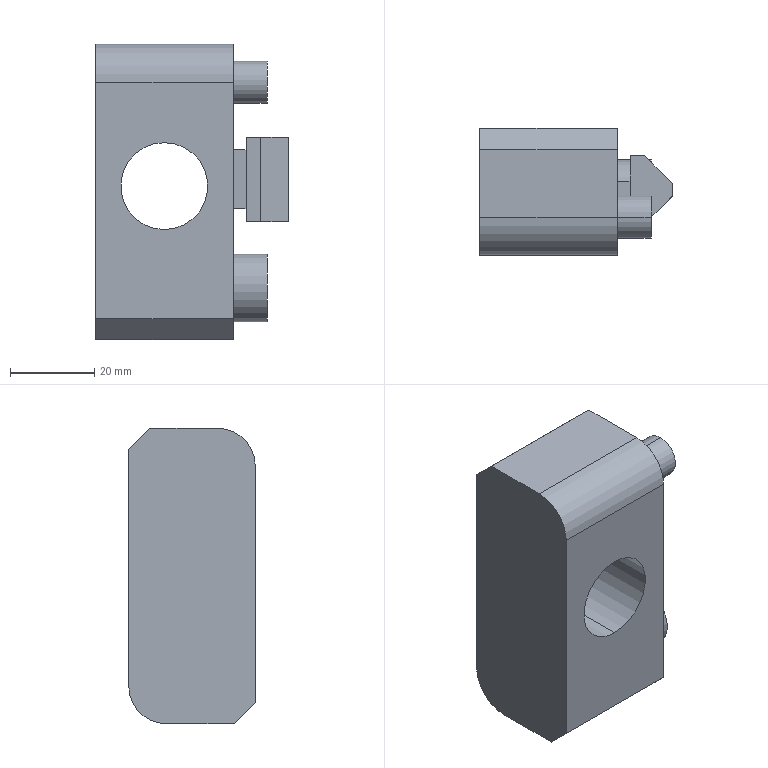Part | SolidWorks | features BaseBody 1 | 1 solid | 30 faces | box 45.6 x 30 x 70 mm | volume 61273 mm3 | plane 22 | cylinder 8 | commonest cylinder face diameters 10 x2 16 x2 18 x2 20.6 x2
STEP:
#1=CARTESIAN_POINT('',(-215.391,-172.8,1136.061));
#2=VERTEX_POINT('',#1);
#3=CARTESIAN_POINT('',(-215.391,-172.8,1126.061));
#4=VERTEX_POINT('',#3);
#5=CARTESIAN_POINT('',(-215.391,-172.8,1131.061));
#6=DIRECTION('',(1.,0.,0.));
#7=DIRECTION('',(0.,0.,-1.));
#8=AXIS2_PLACEMENT_3D('',#5,#6,#7);
#9=CIRCLE('',#8,5.);
#10=EDGE_CURVE('',#2,#4,#9,.T.);
#11=ORIENTED_EDGE('',*,*,#10,.T.);
#12=CARTESIAN_POINT('',(-207.391,-172.8,1126.061));
#13=VERTEX_POINT('',#12);
#14=CARTESIAN_POINT('',(-215.391,-172.8,1126.061));
#15=DIRECTION('',(1.,0.,0.));
#16=VECTOR('',#15,1000.);
#17=LINE('',#14,#16);
#18=EDGE_CURVE('',#4,#13,#17,.T.);
#19=ORIENTED_EDGE('',*,*,#18,.T.);
#20=CARTESIAN_POINT('',(-207.391,-172.8,1136.061));
#21=VERTEX_POINT('',#20);
#22=CARTESIAN_POINT('',(-207.391,-172.8,1131.061));
#23=DIRECTION('',(1.,0.,0.));
#24=DIRECTION('',(0.,-1.,0.));
#25=AXIS2_PLACEMENT_3D('',#22,#23,#24);
#26=CIRCLE('',#25,5.);
#27=EDGE_CURVE('',#21,#13,#26,.T.);
#28=ORIENTED_EDGE('',*,*,#27,.F.);
#29=CARTESIAN_POINT('',(-215.391,-172.8,1136.061));
#30=DIRECTION('',(1.,0.,0.));
#31=VECTOR('',#30,1000.);
#32=LINE('',#29,#31);
#33=EDGE_CURVE('',#2,#21,#32,.T.);
#34=ORIENTED_EDGE('',*,*,#33,.F.);
#35=EDGE_LOOP('',(#11,#19,#28,#34));
#36=FACE_OUTER_BOUND('',#35,.T.);
#37=CARTESIAN_POINT('',(-215.391,-172.8,1131.061));
#38=DIRECTION('',(1.,0.,0.));
#39=DIRECTION('',(0.,0.,1.));
#40=AXIS2_PLACEMENT_3D('',#37,#38,#39);
#41=CYLINDRICAL_SURFACE('',#40,5.);
#42=ADVANCED_FACE('',(#36),#41,.T.);
#43=CARTESIAN_POINT('',(-215.391,-167.047,1090.312));
#44=VERTEX_POINT('',#43);
#45=CARTESIAN_POINT('',(-215.391,-167.047,1074.312));
#46=VERTEX_POINT('',#45);
#47=CARTESIAN_POINT('',(-215.391,-167.047,1082.312));
#48=DIRECTION('',(1.,0.,0.));
#49=DIRECTION('',(0.,-1.,0.));
#50=AXIS2_PLACEMENT_3D('',#47,#48,#49);
#51=CIRCLE('',#50,8.);
#52=EDGE_CURVE('',#44,#46,#51,.T.);
#53=ORIENTED_EDGE('',*,*,#52,.T.);
#54=CARTESIAN_POINT('',(-207.391,-167.047,1074.312));
#55=VERTEX_POINT('',#54);
#56=CARTESIAN_POINT('',(-215.391,-167.047,1074.312));
#57=DIRECTION('',(1.,0.,0.));
#58=VECTOR('',#57,1000.);
#59=LINE('',#56,#58);
#60=EDGE_CURVE('',#46,#55,#59,.T.);
#61=ORIENTED_EDGE('',*,*,#60,.T.);
#62=CARTESIAN_POINT('',(-207.391,-167.047,1090.312));
#63=VERTEX_POINT('',#62);
#64=CARTESIAN_POINT('',(-207.391,-167.047,1082.312));
#65=DIRECTION('',(1.,0.,0.));
#66=DIRECTION('',(0.,-1.,0.));
#67=AXIS2_PLACEMENT_3D('',#64,#65,#66);
#68=CIRCLE('',#67,8.);
#69=EDGE_CURVE('',#63,#55,#68,.T.);
#70=ORIENTED_EDGE('',*,*,#69,.F.);
#71=CARTESIAN_POINT('',(-215.391,-167.047,1090.312));
#72=DIRECTION('',(1.,0.,0.));
#73=VECTOR('',#72,1000.);
#74=LINE('',#71,#73);
#75=EDGE_CURVE('',#44,#63,#74,.T.);
#76=ORIENTED_EDGE('',*,*,#75,.F.);
#77=EDGE_LOOP('',(#53,#61,#70,#76));
#78=FACE_OUTER_BOUND('',#77,.T.);
#79=CARTESIAN_POINT('',(-215.391,-167.047,1082.312));
#80=DIRECTION('',(1.,0.,0.));
#81=DIRECTION('',(0.,0.,1.));
#82=AXIS2_PLACEMENT_3D('',#79,#80,#81);
#83=CYLINDRICAL_SURFACE('',#82,8.);
#84=ADVANCED_FACE('',(#78),#83,.T.);
#85=CARTESIAN_POINT('',(-231.771,-151.8,1096.154));
#86=VERTEX_POINT('',#85);
#87=CARTESIAN_POINT('',(-231.771,-151.8,1116.754));
#88=VERTEX_POINT('',#87);
#89=CARTESIAN_POINT('',(-231.771,-151.8,1106.454));
#90=DIRECTION('',(0.,1.,0.));
#91=DIRECTION('',(-0.8192,0.,0.5736));
#92=AXIS2_PLACEMENT_3D('',#89,#90,#91);
#93=CIRCLE('',#92,10.3);
#94=EDGE_CURVE('',#86,#88,#93,.T.);
#95=ORIENTED_EDGE('',*,*,#94,.T.);
#96=CARTESIAN_POINT('',(-231.771,-181.8,1116.754));
#97=VERTEX_POINT('',#96);
#98=CARTESIAN_POINT('',(-231.771,-151.8,1116.754));
#99=DIRECTION('',(0.,-1.,0.));
#100=VECTOR('',#99,1000.);
#101=LINE('',#98,#100);
#102=EDGE_CURVE('',#88,#97,#101,.T.);
#103=ORIENTED_EDGE('',*,*,#102,.T.);
#104=CARTESIAN_POINT('',(-231.771,-181.8,1096.154));
#105=VERTEX_POINT('',#104);
#106=CARTESIAN_POINT('',(-231.771,-181.8,1106.454));
#107=DIRECTION('',(0.,1.,0.));
#108=DIRECTION('',(-0.8192,0.,0.5736));
#109=AXIS2_PLACEMENT_3D('',#106,#107,#108);
#110=CIRCLE('',#109,10.3);
#111=EDGE_CURVE('',#105,#97,#110,.T.);
#112=ORIENTED_EDGE('',*,*,#111,.F.);
#113=CARTESIAN_POINT('',(-231.771,-151.8,1096.154));
#114=DIRECTION('',(0.,-1.,0.));
#115=VECTOR('',#114,1000.);
#116=LINE('',#113,#115);
#117=EDGE_CURVE('',#86,#105,#116,.T.);
#118=ORIENTED_EDGE('',*,*,#117,.F.);
#119=EDGE_LOOP('',(#95,#103,#112,#118));
#120=FACE_OUTER_BOUND('',#119,.T.);
#121=CARTESIAN_POINT('',(-231.771,-151.8,1106.454));
#122=DIRECTION('',(0.,-1.,0.));
#123=DIRECTION('',(0.,0.,-1.));
#124=AXIS2_PLACEMENT_3D('',#121,#122,#123);
#125=CYLINDRICAL_SURFACE('',#124,10.3);
#126=ADVANCED_FACE('',(#120),#125,.F.);
#127=CARTESIAN_POINT('',(-208.891,-158.258,1098.061));
#128=VERTEX_POINT('',#127);
#129=CARTESIAN_POINT('',(-202.391,-164.758,1098.061));
#130=VERTEX_POINT('',#129);
#131=CARTESIAN_POINT('',(-150.675,-216.475,1098.061));
#132=DIRECTION('',(0.7071,-0.7071,0.));
#133=VECTOR('',#132,1000.);
#134=LINE('',#131,#133);
#135=EDGE_CURVE('',#128,#130,#134,.T.);
#136=ORIENTED_EDGE('',*,*,#135,.F.);
#137=CARTESIAN_POINT('',(-208.891,-158.258,1118.061));
#138=VERTEX_POINT('',#137);
#139=CARTESIAN_POINT('',(-208.891,-158.258,1098.061));
#140=DIRECTION('',(0.,0.,-1.));
#141=VECTOR('',#140,1000.);
#142=LINE('',#139,#141);
#143=EDGE_CURVE('',#138,#128,#142,.T.);
#144=ORIENTED_EDGE('',*,*,#143,.F.);
#145=CARTESIAN_POINT('',(-202.391,-164.758,1118.061));
#146=VERTEX_POINT('',#145);
#147=CARTESIAN_POINT('',(-208.891,-158.258,1118.061));
#148=DIRECTION('',(-0.7071,0.7071,0.));
#149=VECTOR('',#148,1000.);
#150=LINE('',#147,#149);
#151=EDGE_CURVE('',#146,#138,#150,.T.);
#152=ORIENTED_EDGE('',*,*,#151,.F.);
#153=CARTESIAN_POINT('',(-202.391,-164.758,1098.061));
#154=DIRECTION('',(0.,0.,1.));
#155=VECTOR('',#154,1000.);
#156=LINE('',#153,#155);
#157=EDGE_CURVE('',#130,#146,#156,.T.);
#158=ORIENTED_EDGE('',*,*,#157,.F.);
#159=EDGE_LOOP('',(#136,#144,#152,#158));
#160=FACE_OUTER_BOUND('',#159,.T.);
#161=CARTESIAN_POINT('',(-208.891,-158.258,1098.061));
#162=DIRECTION('',(-0.7071,-0.7071,0.));
#163=DIRECTION('',(-0.7071,0.7071,0.));
#164=AXIS2_PLACEMENT_3D('',#161,#162,#163);
#165=PLANE('',#164);
#166=ADVANCED_FACE('',(#160),#165,.F.);
#167=CARTESIAN_POINT('',(-202.391,-167.758,1098.061));
#168=VERTEX_POINT('',#167);
#169=CARTESIAN_POINT('',(-208.891,-174.258,1098.061));
#170=VERTEX_POINT('',#169);
#171=CARTESIAN_POINT('',(-40.216,-5.584,1098.061));
#172=DIRECTION('',(-0.7071,-0.7071,0.));
#173=VECTOR('',#172,1000.);
#174=LINE('',#171,#173);
#175=EDGE_CURVE('',#168,#170,#174,.T.);
#176=ORIENTED_EDGE('',*,*,#175,.F.);
#177=CARTESIAN_POINT('',(-202.391,-167.758,1118.061));
#178=VERTEX_POINT('',#177);
#179=CARTESIAN_POINT('',(-202.391,-167.758,1098.061));
#180=DIRECTION('',(0.,0.,-1.));
#181=VECTOR('',#180,1000.);
#182=LINE('',#179,#181);
#183=EDGE_CURVE('',#178,#168,#182,.T.);
#184=ORIENTED_EDGE('',*,*,#183,.F.);
#185=CARTESIAN_POINT('',(-208.891,-174.258,1118.061));
#186=VERTEX_POINT('',#185);
#187=CARTESIAN_POINT('',(-202.391,-167.758,1118.061));
#188=DIRECTION('',(0.7071,0.7071,0.));
#189=VECTOR('',#188,1000.);
#190=LINE('',#187,#189);
#191=EDGE_CURVE('',#186,#178,#190,.T.);
#192=ORIENTED_EDGE('',*,*,#191,.F.);
#193=CARTESIAN_POINT('',(-208.891,-174.258,1098.061));
#194=DIRECTION('',(0.,0.,1.));
#195=VECTOR('',#194,1000.);
#196=LINE('',#193,#195);
#197=EDGE_CURVE('',#170,#186,#196,.T.);
#198=ORIENTED_EDGE('',*,*,#197,.F.);
#199=EDGE_LOOP('',(#176,#184,#192,#198));
#200=FACE_OUTER_BOUND('',#199,.T.);
#201=CARTESIAN_POINT('',(-202.391,-167.758,1098.061));
#202=DIRECTION('',(-0.7071,0.7071,0.));
#203=DIRECTION('',(0.,0.,1.));
#204=AXIS2_PLACEMENT_3D('',#201,#202,#203);
#205=PLANE('',#204);
#206=ADVANCED_FACE('',(#200),#205,.F.);
#207=CARTESIAN_POINT('',(-215.391,-164.258,1115.061));
#208=VERTEX_POINT('',#207);
#209=CARTESIAN_POINT('',(-212.391,-164.258,1115.061));
#210=VERTEX_POINT('',#209);
#211=CARTESIAN_POINT('',(-212.391,-164.258,1115.061));
#212=DIRECTION('',(1.,0.,0.));
#213=VECTOR('',#212,1000.);
#214=LINE('',#211,#213);
#215=EDGE_CURVE('',#208,#210,#214,.T.);
#216=ORIENTED_EDGE('',*,*,#215,.T.);
#217=CARTESIAN_POINT('',(-212.391,-164.258,1101.061));
#218=VERTEX_POINT('',#217);
#219=CARTESIAN_POINT('',(-212.391,-164.258,1098.061));
#220=DIRECTION('',(0.,0.,-1.));
#221=VECTOR('',#220,1000.);
#222=LINE('',#219,#221);
#223=EDGE_CURVE('',#210,#218,#222,.T.);
#224=ORIENTED_EDGE('',*,*,#223,.T.);
#225=CARTESIAN_POINT('',(-215.391,-164.258,1101.061));
#226=VERTEX_POINT('',#225);
#227=CARTESIAN_POINT('',(-212.391,-164.258,1101.061));
#228=DIRECTION('',(1.,0.,0.));
#229=VECTOR('',#228,1000.);
#230=LINE('',#227,#229);
#231=EDGE_CURVE('',#226,#218,#230,.T.);
#232=ORIENTED_EDGE('',*,*,#231,.F.);
#233=CARTESIAN_POINT('',(-215.391,-164.258,1140.061));
#234=DIRECTION('',(0.,0.,1.));
#235=VECTOR('',#234,1000.);
#236=LINE('',#233,#235);
#237=EDGE_CURVE('',#226,#208,#236,.T.);
#238=ORIENTED_EDGE('',*,*,#237,.T.);
#239=EDGE_LOOP('',(#216,#224,#232,#238));
#240=FACE_OUTER_BOUND('',#239,.T.);
#241=CARTESIAN_POINT('',(-212.391,-164.258,1098.061));
#242=DIRECTION('',(0.,1.,0.));
#243=DIRECTION('',(1.,0.,0.));
#244=AXIS2_PLACEMENT_3D('',#241,#242,#243);
#245=PLANE('',#244);
#246=ADVANCED_FACE('',(#240),#245,.T.);
#247=CARTESIAN_POINT('',(-215.391,-168.258,1101.061));
#248=VERTEX_POINT('',#247);
#249=CARTESIAN_POINT('',(-215.391,-151.8,1101.061));
#250=DIRECTION('',(0.,-1.,0.));
#251=VECTOR('',#250,1000.);
#252=LINE('',#249,#251);
#253=EDGE_CURVE('',#226,#248,#252,.T.);
#254=ORIENTED_EDGE('',*,*,#253,.F.);
#255=ORIENTED_EDGE('',*,*,#231,.T.);
#256=CARTESIAN_POINT('',(-212.391,-168.258,1101.061));
#257=VERTEX_POINT('',#256);
#258=CARTESIAN_POINT('',(-212.391,-158.258,1101.061));
#259=DIRECTION('',(0.,1.,0.));
#260=VECTOR('',#259,1000.);
#261=LINE('',#258,#260);
#262=EDGE_CURVE('',#257,#218,#261,.T.);
#263=ORIENTED_EDGE('',*,*,#262,.F.);
#264=CARTESIAN_POINT('',(-212.391,-168.258,1101.061));
#265=DIRECTION('',(1.,0.,0.));
#266=VECTOR('',#265,1000.);
#267=LINE('',#264,#266);
#268=EDGE_CURVE('',#248,#257,#267,.T.);
#269=ORIENTED_EDGE('',*,*,#268,.F.);
#270=EDGE_LOOP('',(#254,#255,#263,#269));
#271=FACE_OUTER_BOUND('',#270,.T.);
#272=CARTESIAN_POINT('',(-212.391,-158.258,1101.061));
#273=DIRECTION('',(0.,0.,1.));
#274=DIRECTION('',(1.,0.,0.));
#275=AXIS2_PLACEMENT_3D('',#272,#273,#274);
#276=PLANE('',#275);
#277=ADVANCED_FACE('',(#271),#276,.F.);
#278=CARTESIAN_POINT('',(-215.391,-168.258,1115.061));
#279=VERTEX_POINT('',#278);
#280=CARTESIAN_POINT('',(-215.391,-168.258,1140.061));
#281=DIRECTION('',(0.,0.,1.));
#282=VECTOR('',#281,1000.);
#283=LINE('',#280,#282);
#284=EDGE_CURVE('',#248,#279,#283,.T.);
#285=ORIENTED_EDGE('',*,*,#284,.F.);
#286=ORIENTED_EDGE('',*,*,#268,.T.);
#287=CARTESIAN_POINT('',(-212.391,-168.258,1115.061));
#288=VERTEX_POINT('',#287);
#289=CARTESIAN_POINT('',(-212.391,-168.258,1098.061));
#290=DIRECTION('',(0.,0.,-1.));
#291=VECTOR('',#290,1000.);
#292=LINE('',#289,#291);
#293=EDGE_CURVE('',#288,#257,#292,.T.);
#294=ORIENTED_EDGE('',*,*,#293,.F.);
#295=CARTESIAN_POINT('',(-212.391,-168.258,1115.061));
#296=DIRECTION('',(1.,0.,0.));
#297=VECTOR('',#296,1000.);
#298=LINE('',#295,#297);
#299=EDGE_CURVE('',#279,#288,#298,.T.);
#300=ORIENTED_EDGE('',*,*,#299,.F.);
#301=EDGE_LOOP('',(#285,#286,#294,#300));
#302=FACE_OUTER_BOUND('',#301,.T.);
#303=CARTESIAN_POINT('',(-212.391,-168.258,1098.061));
#304=DIRECTION('',(0.,1.,0.));
#305=DIRECTION('',(1.,0.,0.));
#306=AXIS2_PLACEMENT_3D('',#303,#304,#305);
#307=PLANE('',#306);
#308=ADVANCED_FACE('',(#302),#307,.F.);
#309=ORIENTED_EDGE('',*,*,#299,.T.);
#310=CARTESIAN_POINT('',(-212.391,-158.258,1115.061));
#311=DIRECTION('',(0.,1.,0.));
#312=VECTOR('',#311,1000.);
#313=LINE('',#310,#312);
#314=EDGE_CURVE('',#288,#210,#313,.T.);
#315=ORIENTED_EDGE('',*,*,#314,.T.);
#316=ORIENTED_EDGE('',*,*,#215,.F.);
#317=CARTESIAN_POINT('',(-215.391,-151.8,1115.061));
#318=DIRECTION('',(0.,-1.,0.));
#319=VECTOR('',#318,1000.);
#320=LINE('',#317,#319);
#321=EDGE_CURVE('',#208,#279,#320,.T.);
#322=ORIENTED_EDGE('',*,*,#321,.T.);
#323=EDGE_LOOP('',(#309,#315,#316,#322));
#324=FACE_OUTER_BOUND('',#323,.T.);
#325=CARTESIAN_POINT('',(-212.391,-158.258,1115.061));
#326=DIRECTION('',(0.,0.,1.));
#327=DIRECTION('',(1.,0.,0.));
#328=AXIS2_PLACEMENT_3D('',#325,#326,#327);
#329=PLANE('',#328);
#330=ADVANCED_FACE('',(#324),#329,.T.);
#331=CARTESIAN_POINT('',(-202.391,-174.258,1118.061));
#332=DIRECTION('',(0.,-1.,0.));
#333=VECTOR('',#332,1000.);
#334=LINE('',#331,#333);
#335=EDGE_CURVE('',#146,#178,#334,.T.);
#336=ORIENTED_EDGE('',*,*,#335,.F.);
#337=ORIENTED_EDGE('',*,*,#151,.T.);
#338=CARTESIAN_POINT('',(-212.391,-158.258,1118.061));
#339=VERTEX_POINT('',#338);
#340=CARTESIAN_POINT('',(-202.391,-158.258,1118.061));
#341=DIRECTION('',(1.,0.,0.));
#342=VECTOR('',#341,1000.);
#343=LINE('',#340,#342);
#344=EDGE_CURVE('',#339,#138,#343,.T.);
#345=ORIENTED_EDGE('',*,*,#344,.F.);
#346=CARTESIAN_POINT('',(-212.391,-174.258,1118.061));
#347=VERTEX_POINT('',#346);
#348=CARTESIAN_POINT('',(-212.391,-158.258,1118.061));
#349=DIRECTION('',(0.,1.,0.));
#350=VECTOR('',#349,1000.);
#351=LINE('',#348,#350);
#352=EDGE_CURVE('',#347,#339,#351,.T.);
#353=ORIENTED_EDGE('',*,*,#352,.F.);
#354=CARTESIAN_POINT('',(-212.391,-174.258,1118.061));
#355=DIRECTION('',(-1.,0.,0.));
#356=VECTOR('',#355,1000.);
#357=LINE('',#354,#356);
#358=EDGE_CURVE('',#186,#347,#357,.T.);
#359=ORIENTED_EDGE('',*,*,#358,.F.);
#360=ORIENTED_EDGE('',*,*,#191,.T.);
#361=EDGE_LOOP('',(#336,#337,#345,#353,#359,#360));
#362=FACE_OUTER_BOUND('',#361,.T.);
#363=CARTESIAN_POINT('',(10.,-55.8,1118.061));
#364=DIRECTION('',(0.,0.,-1.));
#365=DIRECTION('',(0.,-1.,0.));
#366=AXIS2_PLACEMENT_3D('',#363,#364,#365);
#367=PLANE('',#366);
#368=ADVANCED_FACE('',(#362),#367,.F.);
#369=CARTESIAN_POINT('',(-212.391,-174.258,1098.061));
#370=VERTEX_POINT('',#369);
#371=CARTESIAN_POINT('',(-212.391,-174.258,1098.061));
#372=DIRECTION('',(-1.,0.,0.));
#373=VECTOR('',#372,1000.);
#374=LINE('',#371,#373);
#375=EDGE_CURVE('',#170,#370,#374,.T.);
#376=ORIENTED_EDGE('',*,*,#375,.T.);
#377=CARTESIAN_POINT('',(-212.391,-158.258,1098.061));
#378=VERTEX_POINT('',#377);
#379=CARTESIAN_POINT('',(-212.391,-158.258,1098.061));
#380=DIRECTION('',(0.,1.,0.));
#381=VECTOR('',#380,1000.);
#382=LINE('',#379,#381);
#383=EDGE_CURVE('',#370,#378,#382,.T.);
#384=ORIENTED_EDGE('',*,*,#383,.T.);
#385=CARTESIAN_POINT('',(-202.391,-158.258,1098.061));
#386=DIRECTION('',(1.,0.,0.));
#387=VECTOR('',#386,1000.);
#388=LINE('',#385,#387);
#389=EDGE_CURVE('',#378,#128,#388,.T.);
#390=ORIENTED_EDGE('',*,*,#389,.T.);
#391=ORIENTED_EDGE('',*,*,#135,.T.);
#392=CARTESIAN_POINT('',(-202.391,-174.258,1098.061));
#393=DIRECTION('',(0.,-1.,0.));
#394=VECTOR('',#393,1000.);
#395=LINE('',#392,#394);
#396=EDGE_CURVE('',#130,#168,#395,.T.);
#397=ORIENTED_EDGE('',*,*,#396,.T.);
#398=ORIENTED_EDGE('',*,*,#175,.T.);
#399=EDGE_LOOP('',(#376,#384,#390,#391,#397,#398));
#400=FACE_OUTER_BOUND('',#399,.T.);
#401=CARTESIAN_POINT('',(10.,-55.8,1098.061));
#402=DIRECTION('',(0.,0.,-1.));
#403=DIRECTION('',(0.,-1.,0.));
#404=AXIS2_PLACEMENT_3D('',#401,#402,#403);
#405=PLANE('',#404);
#406=ADVANCED_FACE('',(#400),#405,.T.);
#407=ORIENTED_EDGE('',*,*,#389,.F.);
#408=CARTESIAN_POINT('',(-212.391,-158.258,1098.061));
#409=DIRECTION('',(0.,0.,-1.));
#410=VECTOR('',#409,1000.);
#411=LINE('',#408,#410);
#412=EDGE_CURVE('',#339,#378,#411,.T.);
#413=ORIENTED_EDGE('',*,*,#412,.F.);
#414=ORIENTED_EDGE('',*,*,#344,.T.);
#415=ORIENTED_EDGE('',*,*,#143,.T.);
#416=EDGE_LOOP('',(#407,#413,#414,#415));
#417=FACE_OUTER_BOUND('',#416,.T.);
#418=CARTESIAN_POINT('',(-202.391,-158.258,1098.061));
#419=DIRECTION('',(0.,-1.,0.));
#420=DIRECTION('',(0.,0.,-1.));
#421=AXIS2_PLACEMENT_3D('',#418,#419,#420);
#422=PLANE('',#421);
#423=ADVANCED_FACE('',(#417),#422,.F.);
#424=ORIENTED_EDGE('',*,*,#396,.F.);
#425=ORIENTED_EDGE('',*,*,#157,.T.);
#426=ORIENTED_EDGE('',*,*,#335,.T.);
#427=ORIENTED_EDGE('',*,*,#183,.T.);
#428=EDGE_LOOP('',(#424,#425,#426,#427));
#429=FACE_OUTER_BOUND('',#428,.T.);
#430=CARTESIAN_POINT('',(-202.391,-174.258,1098.061));
#431=DIRECTION('',(-1.,0.,0.));
#432=DIRECTION('',(0.,0.,1.));
#433=AXIS2_PLACEMENT_3D('',#430,#431,#432);
#434=PLANE('',#433);
#435=ADVANCED_FACE('',(#429),#434,.F.);
#436=ORIENTED_EDGE('',*,*,#358,.T.);
#437=CARTESIAN_POINT('',(-212.391,-174.258,1098.061));
#438=DIRECTION('',(0.,0.,-1.));
#439=VECTOR('',#438,1000.);
#440=LINE('',#437,#439);
#441=EDGE_CURVE('',#347,#370,#440,.T.);
#442=ORIENTED_EDGE('',*,*,#441,.T.);
#443=ORIENTED_EDGE('',*,*,#375,.F.);
#444=ORIENTED_EDGE('',*,*,#197,.T.);
#445=EDGE_LOOP('',(#436,#442,#443,#444));
#446=FACE_OUTER_BOUND('',#445,.T.);
#447=CARTESIAN_POINT('',(-212.391,-174.258,1098.061));
#448=DIRECTION('',(0.,1.,0.));
#449=DIRECTION('',(1.,0.,0.));
#450=AXIS2_PLACEMENT_3D('',#447,#448,#449);
#451=PLANE('',#450);
#452=ADVANCED_FACE('',(#446),#451,.F.);
#453=ORIENTED_EDGE('',*,*,#314,.F.);
#454=ORIENTED_EDGE('',*,*,#293,.T.);
#455=ORIENTED_EDGE('',*,*,#262,.T.);
#456=ORIENTED_EDGE('',*,*,#223,.F.);
#457=EDGE_LOOP('',(#453,#454,#455,#456));
#458=FACE_BOUND('',#457,.T.);
#459=ORIENTED_EDGE('',*,*,#352,.T.);
#460=ORIENTED_EDGE('',*,*,#412,.T.);
#461=ORIENTED_EDGE('',*,*,#383,.F.);
#462=ORIENTED_EDGE('',*,*,#441,.F.);
#463=EDGE_LOOP('',(#459,#460,#461,#462));
#464=FACE_OUTER_BOUND('',#463,.T.);
#465=CARTESIAN_POINT('',(-212.391,-158.258,1098.061));
#466=DIRECTION('',(1.,0.,0.));
#467=DIRECTION('',(0.,1.,0.));
#468=AXIS2_PLACEMENT_3D('',#465,#466,#467);
#469=PLANE('',#468);
#470=ADVANCED_FACE('',(#458,#464),#469,.F.);
#471=CARTESIAN_POINT('',(-215.391,-181.8,1075.061));
#472=VERTEX_POINT('',#471);
#473=CARTESIAN_POINT('',(-215.391,-176.8,1070.061));
#474=VERTEX_POINT('',#473);
#475=CARTESIAN_POINT('',(-215.391,-199.3,1092.561));
#476=DIRECTION('',(0.,0.7071,-0.7071));
#477=VECTOR('',#476,1000.);
#478=LINE('',#475,#477);
#479=EDGE_CURVE('',#472,#474,#478,.T.);
#480=ORIENTED_EDGE('',*,*,#479,.F.);
#481=CARTESIAN_POINT('',(-247.991,-181.8,1075.061));
#482=VERTEX_POINT('',#481);
#483=CARTESIAN_POINT('',(-247.991,-181.8,1075.061));
#484=DIRECTION('',(1.,0.,0.));
#485=VECTOR('',#484,1000.);
#486=LINE('',#483,#485);
#487=EDGE_CURVE('',#482,#472,#486,.T.);
#488=ORIENTED_EDGE('',*,*,#487,.F.);
#489=CARTESIAN_POINT('',(-247.991,-176.8,1070.061));
#490=VERTEX_POINT('',#489);
#491=CARTESIAN_POINT('',(-247.991,-164.3,1057.561));
#492=DIRECTION('',(0.,-0.7071,0.7071));
#493=VECTOR('',#492,1000.);
#494=LINE('',#491,#493);
#495=EDGE_CURVE('',#490,#482,#494,.T.);
#496=ORIENTED_EDGE('',*,*,#495,.F.);
#497=CARTESIAN_POINT('',(-215.391,-176.8,1070.061));
#498=DIRECTION('',(-1.,0.,0.));
#499=VECTOR('',#498,1000.);
#500=LINE('',#497,#499);
#501=EDGE_CURVE('',#474,#490,#500,.T.);
#502=ORIENTED_EDGE('',*,*,#501,.F.);
#503=EDGE_LOOP('',(#480,#488,#496,#502));
#504=FACE_OUTER_BOUND('',#503,.T.);
#505=CARTESIAN_POINT('',(-231.771,-181.8,1075.061));
#506=DIRECTION('',(0.,-0.7071,-0.7071));
#507=DIRECTION('',(0.,-0.7071,0.7071));
#508=AXIS2_PLACEMENT_3D('',#505,#506,#507);
#509=PLANE('',#508);
#510=ADVANCED_FACE('',(#504),#509,.T.);
#511=CARTESIAN_POINT('',(-247.991,-156.8,1140.061));
#512=VERTEX_POINT('',#511);
#513=CARTESIAN_POINT('',(-247.991,-151.8,1135.061));
#514=VERTEX_POINT('',#513);
#515=CARTESIAN_POINT('',(-247.991,-119.3,1102.561));
#516=DIRECTION('',(0.,0.7071,-0.7071));
#517=VECTOR('',#516,1000.);
#518=LINE('',#515,#517);
#519=EDGE_CURVE('',#512,#514,#518,.T.);
#520=ORIENTED_EDGE('',*,*,#519,.F.);
#521=CARTESIAN_POINT('',(-215.391,-156.8,1140.061));
#522=VERTEX_POINT('',#521);
#523=CARTESIAN_POINT('',(-247.991,-156.8,1140.061));
#524=DIRECTION('',(-1.,0.,0.));
#525=VECTOR('',#524,1000.);
#526=LINE('',#523,#525);
#527=EDGE_CURVE('',#522,#512,#526,.T.);
#528=ORIENTED_EDGE('',*,*,#527,.F.);
#529=CARTESIAN_POINT('',(-215.391,-151.8,1135.061));
#530=VERTEX_POINT('',#529);
#531=CARTESIAN_POINT('',(-215.391,-154.3,1137.561));
#532=DIRECTION('',(0.,-0.7071,0.7071));
#533=VECTOR('',#532,1000.);
#534=LINE('',#531,#533);
#535=EDGE_CURVE('',#530,#522,#534,.T.);
#536=ORIENTED_EDGE('',*,*,#535,.F.);
#537=CARTESIAN_POINT('',(-231.771,-151.8,1135.061));
#538=DIRECTION('',(1.,0.,0.));
#539=VECTOR('',#538,1000.);
#540=LINE('',#537,#539);
#541=EDGE_CURVE('',#514,#530,#540,.T.);
#542=ORIENTED_EDGE('',*,*,#541,.F.);
#543=EDGE_LOOP('',(#520,#528,#536,#542));
#544=FACE_OUTER_BOUND('',#543,.T.);
#545=CARTESIAN_POINT('',(-247.991,-156.8,1140.061));
#546=DIRECTION('',(0.,-0.7071,-0.7071));
#547=DIRECTION('',(0.,-0.7071,0.7071));
#548=AXIS2_PLACEMENT_3D('',#545,#546,#547);
#549=PLANE('',#548);
#550=ADVANCED_FACE('',(#544),#549,.F.);
#551=ORIENTED_EDGE('',*,*,#27,.T.);
#552=CARTESIAN_POINT('',(-207.391,-172.8,1131.061));
#553=DIRECTION('',(1.,0.,0.));
#554=DIRECTION('',(0.,-1.,0.));
#555=AXIS2_PLACEMENT_3D('',#552,#553,#554);
#556=CIRCLE('',#555,5.);
#557=EDGE_CURVE('',#13,#21,#556,.T.);
#558=ORIENTED_EDGE('',*,*,#557,.T.);
#559=EDGE_LOOP('',(#551,#558));
#560=FACE_OUTER_BOUND('',#559,.T.);
#561=CARTESIAN_POINT('',(-207.391,-172.8,1131.061));
#562=DIRECTION('',(1.,0.,0.));
#563=DIRECTION('',(0.,1.,0.));
#564=AXIS2_PLACEMENT_3D('',#561,#562,#563);
#565=PLANE('',#564);
#566=ADVANCED_FACE('',(#560),#565,.T.);
#567=ORIENTED_EDGE('',*,*,#69,.T.);
#568=CARTESIAN_POINT('',(-207.391,-167.047,1082.312));
#569=DIRECTION('',(1.,0.,0.));
#570=DIRECTION('',(0.,-1.,0.));
#571=AXIS2_PLACEMENT_3D('',#568,#569,#570);
#572=CIRCLE('',#571,8.);
#573=EDGE_CURVE('',#55,#63,#572,.T.);
#574=ORIENTED_EDGE('',*,*,#573,.T.);
#575=EDGE_LOOP('',(#567,#574));
#576=FACE_OUTER_BOUND('',#575,.T.);
#577=CARTESIAN_POINT('',(-207.391,-167.047,1082.312));
#578=DIRECTION('',(1.,0.,0.));
#579=DIRECTION('',(0.,1.,0.));
#580=AXIS2_PLACEMENT_3D('',#577,#578,#579);
#581=PLANE('',#580);
#582=ADVANCED_FACE('',(#576),#581,.T.);
#583=CARTESIAN_POINT('',(-247.991,-181.8,1131.061));
#584=VERTEX_POINT('',#583);
#585=CARTESIAN_POINT('',(-247.991,-172.8,1140.061));
#586=VERTEX_POINT('',#585);
#587=CARTESIAN_POINT('',(-247.991,-172.8,1131.061));
#588=DIRECTION('',(-1.,0.,0.));
#589=DIRECTION('',(0.,0.,1.));
#590=AXIS2_PLACEMENT_3D('',#587,#588,#589);
#591=CIRCLE('',#590,9.);
#592=EDGE_CURVE('',#584,#586,#591,.T.);
#593=ORIENTED_EDGE('',*,*,#592,.F.);
#594=CARTESIAN_POINT('',(-215.391,-181.8,1131.061));
#595=VERTEX_POINT('',#594);
#596=CARTESIAN_POINT('',(-215.391,-181.8,1131.061));
#597=DIRECTION('',(-1.,0.,0.));
#598=VECTOR('',#597,1000.);
#599=LINE('',#596,#598);
#600=EDGE_CURVE('',#595,#584,#599,.T.);
#601=ORIENTED_EDGE('',*,*,#600,.F.);
#602=CARTESIAN_POINT('',(-215.391,-172.8,1140.061));
#603=VERTEX_POINT('',#602);
#604=CARTESIAN_POINT('',(-215.391,-172.8,1131.061));
#605=DIRECTION('',(1.,0.,0.));
#606=DIRECTION('',(0.,0.,-1.));
#607=AXIS2_PLACEMENT_3D('',#604,#605,#606);
#608=CIRCLE('',#607,9.);
#609=EDGE_CURVE('',#603,#595,#608,.T.);
#610=ORIENTED_EDGE('',*,*,#609,.F.);
#611=CARTESIAN_POINT('',(-247.991,-172.8,1140.061));
#612=DIRECTION('',(1.,0.,0.));
#613=VECTOR('',#612,1000.);
#614=LINE('',#611,#613);
#615=EDGE_CURVE('',#586,#603,#614,.T.);
#616=ORIENTED_EDGE('',*,*,#615,.F.);
#617=EDGE_LOOP('',(#593,#601,#610,#616));
#618=FACE_OUTER_BOUND('',#617,.T.);
#619=CARTESIAN_POINT('',(-231.771,-172.8,1131.061));
#620=DIRECTION('',(-1.,0.,0.));
#621=DIRECTION('',(0.,0.,-1.));
#622=AXIS2_PLACEMENT_3D('',#619,#620,#621);
#623=CYLINDRICAL_SURFACE('',#622,9.);
#624=ADVANCED_FACE('',(#618),#623,.T.);
#625=CARTESIAN_POINT('',(-215.391,-160.8,1070.061));
#626=VERTEX_POINT('',#625);
#627=CARTESIAN_POINT('',(-215.391,-151.8,1079.061));
#628=VERTEX_POINT('',#627);
#629=CARTESIAN_POINT('',(-215.391,-160.8,1079.061));
#630=DIRECTION('',(1.,0.,0.));
#631=DIRECTION('',(0.,0.,-1.));
#632=AXIS2_PLACEMENT_3D('',#629,#630,#631);
#633=CIRCLE('',#632,9.);
#634=EDGE_CURVE('',#626,#628,#633,.T.);
#635=ORIENTED_EDGE('',*,*,#634,.F.);
#636=CARTESIAN_POINT('',(-247.991,-160.8,1070.061));
#637=VERTEX_POINT('',#636);
#638=CARTESIAN_POINT('',(-215.391,-160.8,1070.061));
#639=DIRECTION('',(1.,0.,0.));
#640=VECTOR('',#639,1000.);
#641=LINE('',#638,#640);
#642=EDGE_CURVE('',#637,#626,#641,.T.);
#643=ORIENTED_EDGE('',*,*,#642,.F.);
#644=CARTESIAN_POINT('',(-247.991,-151.8,1079.061));
#645=VERTEX_POINT('',#644);
#646=CARTESIAN_POINT('',(-247.991,-160.8,1079.061));
#647=DIRECTION('',(-1.,0.,0.));
#648=DIRECTION('',(0.,0.,1.));
#649=AXIS2_PLACEMENT_3D('',#646,#647,#648);
#650=CIRCLE('',#649,9.);
#651=EDGE_CURVE('',#645,#637,#650,.T.);
#652=ORIENTED_EDGE('',*,*,#651,.F.);
#653=CARTESIAN_POINT('',(-231.771,-151.8,1079.061));
#654=DIRECTION('',(-1.,0.,0.));
#655=VECTOR('',#654,1000.);
#656=LINE('',#653,#655);
#657=EDGE_CURVE('',#628,#645,#656,.T.);
#658=ORIENTED_EDGE('',*,*,#657,.F.);
#659=EDGE_LOOP('',(#635,#643,#652,#658));
#660=FACE_OUTER_BOUND('',#659,.T.);
#661=CARTESIAN_POINT('',(-215.391,-160.8,1079.061));
#662=DIRECTION('',(-1.,0.,0.));
#663=DIRECTION('',(0.,0.,-1.));
#664=AXIS2_PLACEMENT_3D('',#661,#662,#663);
#665=CYLINDRICAL_SURFACE('',#664,9.);
#666=ADVANCED_FACE('',(#660),#665,.T.);
#667=ORIENTED_EDGE('',*,*,#111,.T.);
#668=CARTESIAN_POINT('',(-231.771,-181.8,1106.454));
#669=DIRECTION('',(0.,1.,0.));
#670=DIRECTION('',(-0.8192,0.,0.5736));
#671=AXIS2_PLACEMENT_3D('',#668,#669,#670);
#672=CIRCLE('',#671,10.3);
#673=EDGE_CURVE('',#97,#105,#672,.T.);
#674=ORIENTED_EDGE('',*,*,#673,.T.);
#675=EDGE_LOOP('',(#667,#674));
#676=FACE_BOUND('',#675,.T.);
#677=CARTESIAN_POINT('',(-215.391,-181.8,1140.061));
#678=DIRECTION('',(0.,0.,1.));
#679=VECTOR('',#678,1000.);
#680=LINE('',#677,#679);
#681=EDGE_CURVE('',#472,#595,#680,.T.);
#682=ORIENTED_EDGE('',*,*,#681,.T.);
#683=ORIENTED_EDGE('',*,*,#600,.T.);
#684=CARTESIAN_POINT('',(-247.991,-181.8,1070.061));
#685=DIRECTION('',(0.,0.,-1.));
#686=VECTOR('',#685,1000.);
#687=LINE('',#684,#686);
#688=EDGE_CURVE('',#584,#482,#687,.T.);
#689=ORIENTED_EDGE('',*,*,#688,.T.);
#690=ORIENTED_EDGE('',*,*,#487,.T.);
#691=EDGE_LOOP('',(#682,#683,#689,#690));
#692=FACE_OUTER_BOUND('',#691,.T.);
#693=CARTESIAN_POINT('',(-231.771,-181.8,1106.454));
#694=DIRECTION('',(0.,1.,0.));
#695=DIRECTION('',(1.,0.,0.));
#696=AXIS2_PLACEMENT_3D('',#693,#694,#695);
#697=PLANE('',#696);
#698=ADVANCED_FACE('',(#676,#692),#697,.F.);
#699=ORIENTED_EDGE('',*,*,#94,.F.);
#700=CARTESIAN_POINT('',(-231.771,-151.8,1106.454));
#701=DIRECTION('',(0.,1.,0.));
#702=DIRECTION('',(-0.8192,0.,0.5736));
#703=AXIS2_PLACEMENT_3D('',#700,#701,#702);
#704=CIRCLE('',#703,10.3);
#705=EDGE_CURVE('',#88,#86,#704,.T.);
#706=ORIENTED_EDGE('',*,*,#705,.F.);
#707=EDGE_LOOP('',(#699,#706));
#708=FACE_BOUND('',#707,.T.);
#709=CARTESIAN_POINT('',(-215.391,-151.8,1140.061));
#710=DIRECTION('',(0.,0.,1.));
#711=VECTOR('',#710,1000.);
#712=LINE('',#709,#711);
#713=EDGE_CURVE('',#628,#530,#712,.T.);
#714=ORIENTED_EDGE('',*,*,#713,.F.);
#715=ORIENTED_EDGE('',*,*,#657,.T.);
#716=CARTESIAN_POINT('',(-247.991,-151.8,1070.061));
#717=DIRECTION('',(0.,0.,-1.));
#718=VECTOR('',#717,1000.);
#719=LINE('',#716,#718);
#720=EDGE_CURVE('',#514,#645,#719,.T.);
#721=ORIENTED_EDGE('',*,*,#720,.F.);
#722=ORIENTED_EDGE('',*,*,#541,.T.);
#723=EDGE_LOOP('',(#714,#715,#721,#722));
#724=FACE_OUTER_BOUND('',#723,.T.);
#725=CARTESIAN_POINT('',(-231.771,-151.8,1106.454));
#726=DIRECTION('',(0.,1.,0.));
#727=DIRECTION('',(1.,0.,0.));
#728=AXIS2_PLACEMENT_3D('',#725,#726,#727);
#729=PLANE('',#728);
#730=ADVANCED_FACE('',(#708,#724),#729,.T.);
#731=CARTESIAN_POINT('',(-247.991,-151.8,1070.061));
#732=DIRECTION('',(0.,1.,0.));
#733=VECTOR('',#732,1000.);
#734=LINE('',#731,#733);
#735=EDGE_CURVE('',#490,#637,#734,.T.);
#736=ORIENTED_EDGE('',*,*,#735,.T.);
#737=ORIENTED_EDGE('',*,*,#642,.T.);
#738=CARTESIAN_POINT('',(-215.391,-151.8,1070.061));
#739=DIRECTION('',(0.,1.,0.));
#740=VECTOR('',#739,1000.);
#741=LINE('',#738,#740);
#742=EDGE_CURVE('',#474,#626,#741,.T.);
#743=ORIENTED_EDGE('',*,*,#742,.F.);
#744=ORIENTED_EDGE('',*,*,#501,.T.);
#745=EDGE_LOOP('',(#736,#737,#743,#744));
#746=FACE_OUTER_BOUND('',#745,.T.);
#747=CARTESIAN_POINT('',(-215.391,-151.8,1070.061));
#748=DIRECTION('',(0.,0.,-1.));
#749=DIRECTION('',(0.,-1.,0.));
#750=AXIS2_PLACEMENT_3D('',#747,#748,#749);
#751=PLANE('',#750);
#752=ADVANCED_FACE('',(#746),#751,.T.);
#753=ORIENTED_EDGE('',*,*,#52,.F.);
#754=CARTESIAN_POINT('',(-215.391,-167.047,1082.312));
#755=DIRECTION('',(1.,0.,0.));
#756=DIRECTION('',(0.,-1.,0.));
#757=AXIS2_PLACEMENT_3D('',#754,#755,#756);
#758=CIRCLE('',#757,8.);
#759=EDGE_CURVE('',#46,#44,#758,.T.);
#760=ORIENTED_EDGE('',*,*,#759,.F.);
#761=EDGE_LOOP('',(#753,#760));
#762=FACE_BOUND('',#761,.T.);
#763=ORIENTED_EDGE('',*,*,#10,.F.);
#764=CARTESIAN_POINT('',(-215.391,-172.8,1131.061));
#765=DIRECTION('',(1.,0.,0.));
#766=DIRECTION('',(0.,0.,-1.));
#767=AXIS2_PLACEMENT_3D('',#764,#765,#766);
#768=CIRCLE('',#767,5.);
#769=EDGE_CURVE('',#4,#2,#768,.T.);
#770=ORIENTED_EDGE('',*,*,#769,.F.);
#771=EDGE_LOOP('',(#763,#770));
#772=FACE_BOUND('',#771,.T.);
#773=ORIENTED_EDGE('',*,*,#321,.F.);
#774=ORIENTED_EDGE('',*,*,#237,.F.);
#775=ORIENTED_EDGE('',*,*,#253,.T.);
#776=ORIENTED_EDGE('',*,*,#284,.T.);
#777=EDGE_LOOP('',(#773,#774,#775,#776));
#778=FACE_BOUND('',#777,.T.);
#779=CARTESIAN_POINT('',(-215.391,-151.8,1140.061));
#780=DIRECTION('',(0.,1.,0.));
#781=VECTOR('',#780,1000.);
#782=LINE('',#779,#781);
#783=EDGE_CURVE('',#603,#522,#782,.T.);
#784=ORIENTED_EDGE('',*,*,#783,.F.);
#785=ORIENTED_EDGE('',*,*,#609,.T.);
#786=ORIENTED_EDGE('',*,*,#681,.F.);
#787=ORIENTED_EDGE('',*,*,#479,.T.);
#788=ORIENTED_EDGE('',*,*,#742,.T.);
#789=ORIENTED_EDGE('',*,*,#634,.T.);
#790=ORIENTED_EDGE('',*,*,#713,.T.);
#791=ORIENTED_EDGE('',*,*,#535,.T.);
#792=EDGE_LOOP('',(#784,#785,#786,#787,#788,#789,#790,#791));
#793=FACE_OUTER_BOUND('',#792,.T.);
#794=CARTESIAN_POINT('',(-215.391,-151.8,1140.061));
#795=DIRECTION('',(1.,0.,0.));
#796=DIRECTION('',(0.,1.,0.));
#797=AXIS2_PLACEMENT_3D('',#794,#795,#796);
#798=PLANE('',#797);
#799=ADVANCED_FACE('',(#762,#772,#778,#793),#798,.T.);
#800=CARTESIAN_POINT('',(-247.991,-151.8,1140.061));
#801=DIRECTION('',(0.,1.,0.));
#802=VECTOR('',#801,1000.);
#803=LINE('',#800,#802);
#804=EDGE_CURVE('',#586,#512,#803,.T.);
#805=ORIENTED_EDGE('',*,*,#804,.F.);
#806=ORIENTED_EDGE('',*,*,#615,.T.);
#807=ORIENTED_EDGE('',*,*,#783,.T.);
#808=ORIENTED_EDGE('',*,*,#527,.T.);
#809=EDGE_LOOP('',(#805,#806,#807,#808));
#810=FACE_OUTER_BOUND('',#809,.T.);
#811=CARTESIAN_POINT('',(-247.991,-151.8,1140.061));
#812=DIRECTION('',(0.,0.,1.));
#813=DIRECTION('',(1.,0.,0.));
#814=AXIS2_PLACEMENT_3D('',#811,#812,#813);
#815=PLANE('',#814);
#816=ADVANCED_FACE('',(#810),#815,.T.);
#817=ORIENTED_EDGE('',*,*,#720,.T.);
#818=ORIENTED_EDGE('',*,*,#651,.T.);
#819=ORIENTED_EDGE('',*,*,#735,.F.);
#820=ORIENTED_EDGE('',*,*,#495,.T.);
#821=ORIENTED_EDGE('',*,*,#688,.F.);
#822=ORIENTED_EDGE('',*,*,#592,.T.);
#823=ORIENTED_EDGE('',*,*,#804,.T.);
#824=ORIENTED_EDGE('',*,*,#519,.T.);
#825=EDGE_LOOP('',(#817,#818,#819,#820,#821,#822,#823,#824));
#826=FACE_OUTER_BOUND('',#825,.T.);
#827=CARTESIAN_POINT('',(-247.991,-151.8,1070.061));
#828=DIRECTION('',(-1.,0.,0.));
#829=DIRECTION('',(0.,0.,1.));
#830=AXIS2_PLACEMENT_3D('',#827,#828,#829);
#831=PLANE('',#830);
#832=ADVANCED_FACE('',(#826),#831,.T.);
#833=ORIENTED_EDGE('',*,*,#102,.F.);
#834=ORIENTED_EDGE('',*,*,#705,.T.);
#835=ORIENTED_EDGE('',*,*,#117,.T.);
#836=ORIENTED_EDGE('',*,*,#673,.F.);
#837=EDGE_LOOP('',(#833,#834,#835,#836));
#838=FACE_OUTER_BOUND('',#837,.T.);
#839=CARTESIAN_POINT('',(-231.771,-151.8,1106.454));
#840=DIRECTION('',(0.,-1.,0.));
#841=DIRECTION('',(0.,0.,-1.));
#842=AXIS2_PLACEMENT_3D('',#839,#840,#841);
#843=CYLINDRICAL_SURFACE('',#842,10.3);
#844=ADVANCED_FACE('',(#838),#843,.F.);
#845=ORIENTED_EDGE('',*,*,#60,.F.);
#846=ORIENTED_EDGE('',*,*,#759,.T.);
#847=ORIENTED_EDGE('',*,*,#75,.T.);
#848=ORIENTED_EDGE('',*,*,#573,.F.);
#849=EDGE_LOOP('',(#845,#846,#847,#848));
#850=FACE_OUTER_BOUND('',#849,.T.);
#851=CARTESIAN_POINT('',(-215.391,-167.047,1082.312));
#852=DIRECTION('',(1.,0.,0.));
#853=DIRECTION('',(0.,0.,1.));
#854=AXIS2_PLACEMENT_3D('',#851,#852,#853);
#855=CYLINDRICAL_SURFACE('',#854,8.);
#856=ADVANCED_FACE('',(#850),#855,.T.);
#857=ORIENTED_EDGE('',*,*,#18,.F.);
#858=ORIENTED_EDGE('',*,*,#769,.T.);
#859=ORIENTED_EDGE('',*,*,#33,.T.);
#860=ORIENTED_EDGE('',*,*,#557,.F.);
#861=EDGE_LOOP('',(#857,#858,#859,#860));
#862=FACE_OUTER_BOUND('',#861,.T.);
#863=CARTESIAN_POINT('',(-215.391,-172.8,1131.061));
#864=DIRECTION('',(1.,0.,0.));
#865=DIRECTION('',(0.,0.,1.));
#866=AXIS2_PLACEMENT_3D('',#863,#864,#865);
#867=CYLINDRICAL_SURFACE('',#866,5.);
#868=ADVANCED_FACE('',(#862),#867,.T.);
#869=CLOSED_SHELL('',(#42,#84,#126,#166,#206,#246,#277,#308,#330,#368,#406,#423,#435,#452,#470,#510,#550,#566,#582,#624,#666,#698,#730,#752,#799,#816,#832,#844,#856,#868));
#870=MANIFOLD_SOLID_BREP('',#869);
#871=CARTESIAN_POINT('',(0.,0.,0.));
#872=DIRECTION('',(0.,0.,1.));
#873=DIRECTION('',(1.,0.,0.));
#874=AXIS2_PLACEMENT_3D('',#871,#872,#873);
#875=(LENGTH_UNIT()NAMED_UNIT(*)SI_UNIT(.MILLI.,.METRE.));
#876=UNCERTAINTY_MEASURE_WITH_UNIT(LENGTH_MEASURE(0.00001),#875,'','');
#877=(NAMED_UNIT(*)PLANE_ANGLE_UNIT()SI_UNIT($,.RADIAN.));
#878=(NAMED_UNIT(*)SI_UNIT($,.STERADIAN.)SOLID_ANGLE_UNIT());
#879=(GEOMETRIC_REPRESENTATION_CONTEXT(3)GLOBAL_UNCERTAINTY_ASSIGNED_CONTEXT((#876))GLOBAL_UNIT_ASSIGNED_CONTEXT((#875,#877,#878))REPRESENTATION_CONTEXT('',''));
#880=ADVANCED_BREP_SHAPE_REPRESENTATION('',(#870,#874),#879);